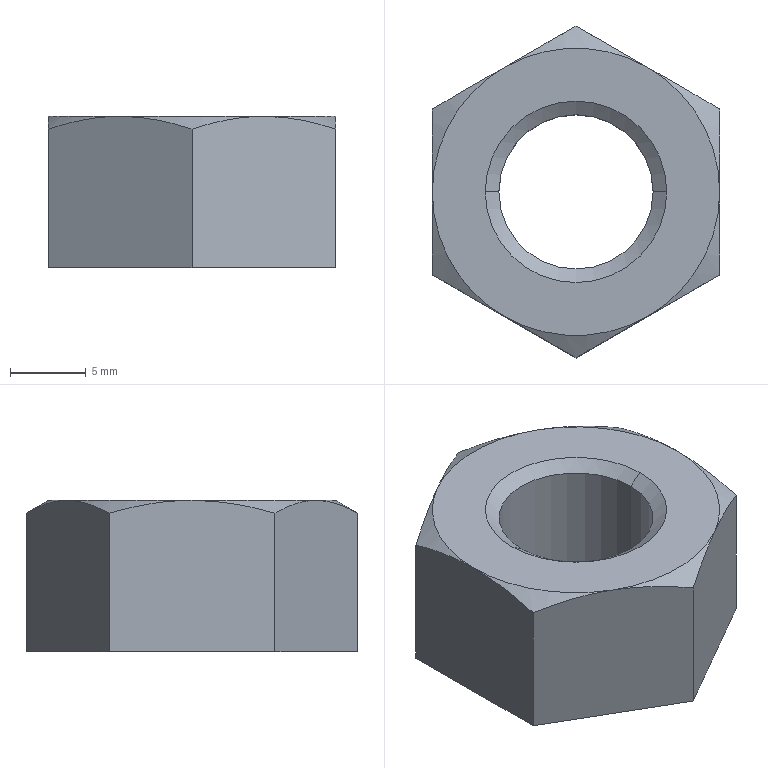Part | STEP file | PN_0064_hex nut-M12x1.75 | 1 solid | 22 faces | box 19 x 21.939 x 10 mm | volume 2282 mm3 | cone 10 | plane 8 | cylinder 4 | commonest cylinder face diameters 10.2 x2 12 x2